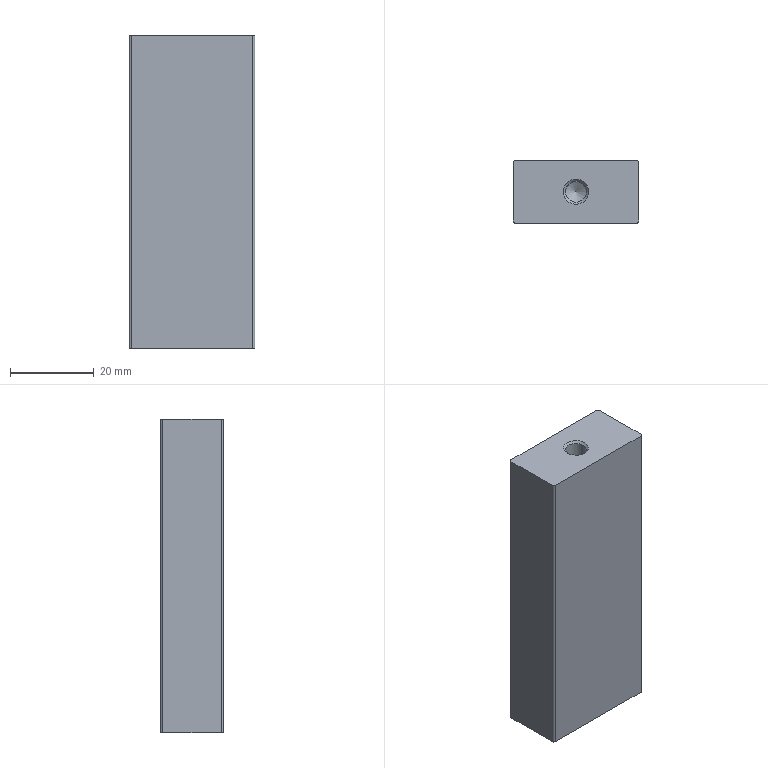Part | STEP file | 200 mesh_id1938 | 1 solid | 13 faces | box 30 x 15 x 75 mm | volume 33075 mm3 | plane 6 | cylinder 5 | cone 2 | commonest cylinder face diameters 1 x4 5 x1
STEP:
#1=CARTESIAN_POINT('',(-16621.224,-4110.769,87.));
#2=VERTEX_POINT('',#1);
#3=CARTESIAN_POINT('',(-16621.224,-4124.769,87.));
#4=VERTEX_POINT('',#3);
#5=CARTESIAN_POINT('',(-16621.224,-4110.769,87.));
#6=DIRECTION('',(0.,-1.,0.));
#7=VECTOR('',#6,1.);
#8=LINE('',#5,#7);
#9=EDGE_CURVE('',#2,#4,#8,.T.);
#10=ORIENTED_EDGE('',*,*,#9,.T.);
#11=CARTESIAN_POINT('',(-16621.224,-4124.769,12.));
#12=VERTEX_POINT('',#11);
#13=CARTESIAN_POINT('',(-16621.224,-4124.769,12.));
#14=DIRECTION('',(0.,0.,1.));
#15=VECTOR('',#14,1.);
#16=LINE('',#13,#15);
#17=EDGE_CURVE('',#12,#4,#16,.T.);
#18=ORIENTED_EDGE('',*,*,#17,.F.);
#19=CARTESIAN_POINT('',(-16621.224,-4110.769,12.));
#20=VERTEX_POINT('',#19);
#21=CARTESIAN_POINT('',(-16621.224,-4110.769,12.));
#22=DIRECTION('',(0.,-1.,0.));
#23=VECTOR('',#22,1.);
#24=LINE('',#21,#23);
#25=EDGE_CURVE('',#20,#12,#24,.T.);
#26=ORIENTED_EDGE('',*,*,#25,.F.);
#27=CARTESIAN_POINT('',(-16621.224,-4110.769,12.));
#28=DIRECTION('',(0.,0.,1.));
#29=VECTOR('',#28,1.);
#30=LINE('',#27,#29);
#31=EDGE_CURVE('',#20,#2,#30,.T.);
#32=ORIENTED_EDGE('',*,*,#31,.T.);
#33=EDGE_LOOP('',(#10,#18,#26,#32));
#34=FACE_OUTER_BOUND('',#33,.T.);
#35=CARTESIAN_POINT('',(-16621.224,-4110.769,12.));
#36=DIRECTION('',(-1.,0.,0.));
#37=DIRECTION('',(0.,-1.,0.));
#38=AXIS2_PLACEMENT_3D('',#35,#36,#37);
#39=PLANE('',#38);
#40=ADVANCED_FACE('',(#34),#39,.F.);
#41=CARTESIAN_POINT('',(-16621.724,-4125.269,87.));
#42=VERTEX_POINT('',#41);
#43=CARTESIAN_POINT('',(-16621.724,-4124.769,87.));
#44=DIRECTION('',(0.,0.,-1.));
#45=DIRECTION('',(1.,0.,0.));
#46=AXIS2_PLACEMENT_3D('',#43,#44,#45);
#47=CIRCLE('',#46,0.5);
#48=EDGE_CURVE('',#4,#42,#47,.T.);
#49=ORIENTED_EDGE('',*,*,#48,.T.);
#50=CARTESIAN_POINT('',(-16621.724,-4125.269,12.));
#51=VERTEX_POINT('',#50);
#52=CARTESIAN_POINT('',(-16621.724,-4125.269,12.));
#53=DIRECTION('',(0.,0.,1.));
#54=VECTOR('',#53,1.);
#55=LINE('',#52,#54);
#56=EDGE_CURVE('',#51,#42,#55,.T.);
#57=ORIENTED_EDGE('',*,*,#56,.F.);
#58=CARTESIAN_POINT('',(-16621.724,-4124.769,12.));
#59=DIRECTION('',(0.,0.,-1.));
#60=DIRECTION('',(1.,0.,0.));
#61=AXIS2_PLACEMENT_3D('',#58,#59,#60);
#62=CIRCLE('',#61,0.5);
#63=EDGE_CURVE('',#12,#51,#62,.T.);
#64=ORIENTED_EDGE('',*,*,#63,.F.);
#65=ORIENTED_EDGE('',*,*,#17,.T.);
#66=EDGE_LOOP('',(#49,#57,#64,#65));
#67=FACE_OUTER_BOUND('',#66,.T.);
#68=CARTESIAN_POINT('',(-16621.724,-4124.769,12.));
#69=DIRECTION('',(0.,0.,1.));
#70=DIRECTION('',(1.,0.,0.));
#71=AXIS2_PLACEMENT_3D('',#68,#69,#70);
#72=CYLINDRICAL_SURFACE('',#71,0.5);
#73=ADVANCED_FACE('',(#67),#72,.T.);
#74=CARTESIAN_POINT('',(-16650.724,-4125.269,87.));
#75=VERTEX_POINT('',#74);
#76=CARTESIAN_POINT('',(-16621.724,-4125.269,87.));
#77=DIRECTION('',(-1.,0.,0.));
#78=VECTOR('',#77,1.);
#79=LINE('',#76,#78);
#80=EDGE_CURVE('',#42,#75,#79,.T.);
#81=ORIENTED_EDGE('',*,*,#80,.T.);
#82=CARTESIAN_POINT('',(-16650.724,-4125.269,12.));
#83=VERTEX_POINT('',#82);
#84=CARTESIAN_POINT('',(-16650.724,-4125.269,12.));
#85=DIRECTION('',(0.,0.,1.));
#86=VECTOR('',#85,1.);
#87=LINE('',#84,#86);
#88=EDGE_CURVE('',#83,#75,#87,.T.);
#89=ORIENTED_EDGE('',*,*,#88,.F.);
#90=CARTESIAN_POINT('',(-16621.724,-4125.269,12.));
#91=DIRECTION('',(-1.,0.,0.));
#92=VECTOR('',#91,1.);
#93=LINE('',#90,#92);
#94=EDGE_CURVE('',#51,#83,#93,.T.);
#95=ORIENTED_EDGE('',*,*,#94,.F.);
#96=ORIENTED_EDGE('',*,*,#56,.T.);
#97=EDGE_LOOP('',(#81,#89,#95,#96));
#98=FACE_OUTER_BOUND('',#97,.T.);
#99=CARTESIAN_POINT('',(-16621.724,-4125.269,12.));
#100=DIRECTION('',(0.,1.,0.));
#101=DIRECTION('',(0.,0.,1.));
#102=AXIS2_PLACEMENT_3D('',#99,#100,#101);
#103=PLANE('',#102);
#104=ADVANCED_FACE('',(#98),#103,.F.);
#105=CARTESIAN_POINT('',(-16651.224,-4124.769,87.));
#106=VERTEX_POINT('',#105);
#107=CARTESIAN_POINT('',(-16650.724,-4124.769,87.));
#108=DIRECTION('',(0.,0.,-1.));
#109=DIRECTION('',(1.,0.,0.));
#110=AXIS2_PLACEMENT_3D('',#107,#108,#109);
#111=CIRCLE('',#110,0.5);
#112=EDGE_CURVE('',#75,#106,#111,.T.);
#113=ORIENTED_EDGE('',*,*,#112,.T.);
#114=CARTESIAN_POINT('',(-16651.224,-4124.769,12.));
#115=VERTEX_POINT('',#114);
#116=CARTESIAN_POINT('',(-16651.224,-4124.769,12.));
#117=DIRECTION('',(0.,0.,1.));
#118=VECTOR('',#117,1.);
#119=LINE('',#116,#118);
#120=EDGE_CURVE('',#115,#106,#119,.T.);
#121=ORIENTED_EDGE('',*,*,#120,.F.);
#122=CARTESIAN_POINT('',(-16650.724,-4124.769,12.));
#123=DIRECTION('',(0.,0.,-1.));
#124=DIRECTION('',(1.,0.,0.));
#125=AXIS2_PLACEMENT_3D('',#122,#123,#124);
#126=CIRCLE('',#125,0.5);
#127=EDGE_CURVE('',#83,#115,#126,.T.);
#128=ORIENTED_EDGE('',*,*,#127,.F.);
#129=ORIENTED_EDGE('',*,*,#88,.T.);
#130=EDGE_LOOP('',(#113,#121,#128,#129));
#131=FACE_OUTER_BOUND('',#130,.T.);
#132=CARTESIAN_POINT('',(-16650.724,-4124.769,12.));
#133=DIRECTION('',(0.,0.,1.));
#134=DIRECTION('',(1.,0.,0.));
#135=AXIS2_PLACEMENT_3D('',#132,#133,#134);
#136=CYLINDRICAL_SURFACE('',#135,0.5);
#137=ADVANCED_FACE('',(#131),#136,.T.);
#138=CARTESIAN_POINT('',(-16651.224,-4110.769,87.));
#139=VERTEX_POINT('',#138);
#140=CARTESIAN_POINT('',(-16651.224,-4124.769,87.));
#141=DIRECTION('',(0.,1.,0.));
#142=VECTOR('',#141,1.);
#143=LINE('',#140,#142);
#144=EDGE_CURVE('',#106,#139,#143,.T.);
#145=ORIENTED_EDGE('',*,*,#144,.T.);
#146=CARTESIAN_POINT('',(-16651.224,-4110.769,12.));
#147=VERTEX_POINT('',#146);
#148=CARTESIAN_POINT('',(-16651.224,-4110.769,12.));
#149=DIRECTION('',(0.,0.,1.));
#150=VECTOR('',#149,1.);
#151=LINE('',#148,#150);
#152=EDGE_CURVE('',#147,#139,#151,.T.);
#153=ORIENTED_EDGE('',*,*,#152,.F.);
#154=CARTESIAN_POINT('',(-16651.224,-4124.769,12.));
#155=DIRECTION('',(0.,1.,0.));
#156=VECTOR('',#155,1.);
#157=LINE('',#154,#156);
#158=EDGE_CURVE('',#115,#147,#157,.T.);
#159=ORIENTED_EDGE('',*,*,#158,.F.);
#160=ORIENTED_EDGE('',*,*,#120,.T.);
#161=EDGE_LOOP('',(#145,#153,#159,#160));
#162=FACE_OUTER_BOUND('',#161,.T.);
#163=CARTESIAN_POINT('',(-16651.224,-4124.769,12.));
#164=DIRECTION('',(1.,0.,0.));
#165=DIRECTION('',(0.,0.,-1.));
#166=AXIS2_PLACEMENT_3D('',#163,#164,#165);
#167=PLANE('',#166);
#168=ADVANCED_FACE('',(#162),#167,.F.);
#169=CARTESIAN_POINT('',(-16650.724,-4110.269,87.));
#170=VERTEX_POINT('',#169);
#171=CARTESIAN_POINT('',(-16650.724,-4110.769,87.));
#172=DIRECTION('',(0.,0.,-1.));
#173=DIRECTION('',(1.,0.,0.));
#174=AXIS2_PLACEMENT_3D('',#171,#172,#173);
#175=CIRCLE('',#174,0.5);
#176=EDGE_CURVE('',#139,#170,#175,.T.);
#177=ORIENTED_EDGE('',*,*,#176,.T.);
#178=CARTESIAN_POINT('',(-16650.724,-4110.269,12.));
#179=VERTEX_POINT('',#178);
#180=CARTESIAN_POINT('',(-16650.724,-4110.269,12.));
#181=DIRECTION('',(0.,0.,1.));
#182=VECTOR('',#181,1.);
#183=LINE('',#180,#182);
#184=EDGE_CURVE('',#179,#170,#183,.T.);
#185=ORIENTED_EDGE('',*,*,#184,.F.);
#186=CARTESIAN_POINT('',(-16650.724,-4110.769,12.));
#187=DIRECTION('',(0.,0.,-1.));
#188=DIRECTION('',(1.,0.,0.));
#189=AXIS2_PLACEMENT_3D('',#186,#187,#188);
#190=CIRCLE('',#189,0.5);
#191=EDGE_CURVE('',#147,#179,#190,.T.);
#192=ORIENTED_EDGE('',*,*,#191,.F.);
#193=ORIENTED_EDGE('',*,*,#152,.T.);
#194=EDGE_LOOP('',(#177,#185,#192,#193));
#195=FACE_OUTER_BOUND('',#194,.T.);
#196=CARTESIAN_POINT('',(-16650.724,-4110.769,12.));
#197=DIRECTION('',(0.,0.,1.));
#198=DIRECTION('',(1.,0.,0.));
#199=AXIS2_PLACEMENT_3D('',#196,#197,#198);
#200=CYLINDRICAL_SURFACE('',#199,0.5);
#201=ADVANCED_FACE('',(#195),#200,.T.);
#202=CARTESIAN_POINT('',(-16621.724,-4110.269,87.));
#203=VERTEX_POINT('',#202);
#204=CARTESIAN_POINT('',(-16650.724,-4110.269,87.));
#205=DIRECTION('',(1.,0.,0.));
#206=VECTOR('',#205,1.);
#207=LINE('',#204,#206);
#208=EDGE_CURVE('',#170,#203,#207,.T.);
#209=ORIENTED_EDGE('',*,*,#208,.T.);
#210=CARTESIAN_POINT('',(-16621.724,-4110.269,12.));
#211=VERTEX_POINT('',#210);
#212=CARTESIAN_POINT('',(-16621.724,-4110.269,12.));
#213=DIRECTION('',(0.,0.,1.));
#214=VECTOR('',#213,1.);
#215=LINE('',#212,#214);
#216=EDGE_CURVE('',#211,#203,#215,.T.);
#217=ORIENTED_EDGE('',*,*,#216,.F.);
#218=CARTESIAN_POINT('',(-16650.724,-4110.269,12.));
#219=DIRECTION('',(1.,0.,0.));
#220=VECTOR('',#219,1.);
#221=LINE('',#218,#220);
#222=EDGE_CURVE('',#179,#211,#221,.T.);
#223=ORIENTED_EDGE('',*,*,#222,.F.);
#224=ORIENTED_EDGE('',*,*,#184,.T.);
#225=EDGE_LOOP('',(#209,#217,#223,#224));
#226=FACE_OUTER_BOUND('',#225,.T.);
#227=CARTESIAN_POINT('',(-16650.724,-4110.269,12.));
#228=DIRECTION('',(0.,-1.,0.));
#229=DIRECTION('',(0.,0.,-1.));
#230=AXIS2_PLACEMENT_3D('',#227,#228,#229);
#231=PLANE('',#230);
#232=ADVANCED_FACE('',(#226),#231,.F.);
#233=CARTESIAN_POINT('',(-16621.724,-4110.769,87.));
#234=DIRECTION('',(0.,0.,-1.));
#235=DIRECTION('',(1.,0.,0.));
#236=AXIS2_PLACEMENT_3D('',#233,#234,#235);
#237=CIRCLE('',#236,0.5);
#238=EDGE_CURVE('',#203,#2,#237,.T.);
#239=ORIENTED_EDGE('',*,*,#238,.T.);
#240=ORIENTED_EDGE('',*,*,#31,.F.);
#241=CARTESIAN_POINT('',(-16621.724,-4110.769,12.));
#242=DIRECTION('',(0.,0.,-1.));
#243=DIRECTION('',(1.,0.,0.));
#244=AXIS2_PLACEMENT_3D('',#241,#242,#243);
#245=CIRCLE('',#244,0.5);
#246=EDGE_CURVE('',#211,#20,#245,.T.);
#247=ORIENTED_EDGE('',*,*,#246,.F.);
#248=ORIENTED_EDGE('',*,*,#216,.T.);
#249=EDGE_LOOP('',(#239,#240,#247,#248));
#250=FACE_OUTER_BOUND('',#249,.T.);
#251=CARTESIAN_POINT('',(-16621.724,-4110.769,12.));
#252=DIRECTION('',(0.,0.,1.));
#253=DIRECTION('',(1.,0.,0.));
#254=AXIS2_PLACEMENT_3D('',#251,#252,#253);
#255=CYLINDRICAL_SURFACE('',#254,0.5);
#256=ADVANCED_FACE('',(#250),#255,.T.);
#257=ORIENTED_EDGE('',*,*,#25,.T.);
#258=ORIENTED_EDGE('',*,*,#63,.T.);
#259=ORIENTED_EDGE('',*,*,#94,.T.);
#260=ORIENTED_EDGE('',*,*,#127,.T.);
#261=ORIENTED_EDGE('',*,*,#158,.T.);
#262=ORIENTED_EDGE('',*,*,#191,.T.);
#263=ORIENTED_EDGE('',*,*,#222,.T.);
#264=ORIENTED_EDGE('',*,*,#246,.T.);
#265=EDGE_LOOP('',(#257,#258,#259,#260,#261,#262,#263,#264));
#266=FACE_OUTER_BOUND('',#265,.T.);
#267=CARTESIAN_POINT('',(-16621.724,-4124.769,12.));
#268=DIRECTION('',(0.,0.,-1.));
#269=DIRECTION('',(-1.,0.,0.));
#270=AXIS2_PLACEMENT_3D('',#267,#268,#269);
#271=PLANE('',#270);
#272=ADVANCED_FACE('',(#266),#271,.T.);
#273=CARTESIAN_POINT('',(-16639.224,-4117.769,87.));
#274=VERTEX_POINT('',#273);
#275=CARTESIAN_POINT('',(-16636.224,-4117.769,87.));
#276=DIRECTION('',(0.,0.,-1.));
#277=DIRECTION('',(-1.,0.,0.));
#278=AXIS2_PLACEMENT_3D('',#275,#276,#277);
#279=CIRCLE('',#278,3.);
#280=EDGE_CURVE('',#274,#274,#279,.T.);
#281=ORIENTED_EDGE('',*,*,#280,.T.);
#282=EDGE_LOOP('',(#281));
#283=FACE_BOUND('',#282,.T.);
#284=ORIENTED_EDGE('',*,*,#9,.F.);
#285=ORIENTED_EDGE('',*,*,#238,.F.);
#286=ORIENTED_EDGE('',*,*,#208,.F.);
#287=ORIENTED_EDGE('',*,*,#176,.F.);
#288=ORIENTED_EDGE('',*,*,#144,.F.);
#289=ORIENTED_EDGE('',*,*,#112,.F.);
#290=ORIENTED_EDGE('',*,*,#80,.F.);
#291=ORIENTED_EDGE('',*,*,#48,.F.);
#292=EDGE_LOOP('',(#284,#285,#286,#287,#288,#289,#290,#291));
#293=FACE_BOUND('',#292,.T.);
#294=CARTESIAN_POINT('',(-16621.724,-4124.769,87.));
#295=DIRECTION('',(0.,0.,-1.));
#296=DIRECTION('',(-1.,0.,0.));
#297=AXIS2_PLACEMENT_3D('',#294,#295,#296);
#298=PLANE('',#297);
#299=ADVANCED_FACE('',(#283,#293),#298,.F.);
#300=CARTESIAN_POINT('',(-16638.724,-4117.769,54.056));
#301=VERTEX_POINT('',#300);
#302=CARTESIAN_POINT('',(-16636.224,-4117.769,54.056));
#303=DIRECTION('',(0.,0.,1.));
#304=DIRECTION('',(-1.,0.,0.));
#305=AXIS2_PLACEMENT_3D('',#302,#303,#304);
#306=CIRCLE('',#305,2.5);
#307=EDGE_CURVE('',#301,#301,#306,.T.);
#308=ORIENTED_EDGE('',*,*,#307,.T.);
#309=EDGE_LOOP('',(#308));
#310=FACE_BOUND('',#309,.T.);
#311=CARTESIAN_POINT('',(-16636.224,-4117.769,52.554));
#312=VERTEX_POINT('',#311);
#313=VERTEX_LOOP('',#312);
#314=FACE_BOUND('',#313,.T.);
#315=CARTESIAN_POINT('',(-16636.224,-4117.769,54.056));
#316=DIRECTION('',(0.,0.,1.));
#317=DIRECTION('',(1.,0.,0.));
#318=AXIS2_PLACEMENT_3D('',#315,#316,#317);
#319=CONICAL_SURFACE('',#318,2.5,59.);
#320=ADVANCED_FACE('',(#310,#314),#319,.F.);
#321=CARTESIAN_POINT('',(-16638.724,-4117.769,86.5));
#322=VERTEX_POINT('',#321);
#323=CARTESIAN_POINT('',(-16636.224,-4117.769,86.5));
#324=DIRECTION('',(0.,0.,1.));
#325=DIRECTION('',(-1.,0.,0.));
#326=AXIS2_PLACEMENT_3D('',#323,#324,#325);
#327=CIRCLE('',#326,2.5);
#328=EDGE_CURVE('',#322,#322,#327,.T.);
#329=ORIENTED_EDGE('',*,*,#328,.T.);
#330=EDGE_LOOP('',(#329));
#331=FACE_BOUND('',#330,.T.);
#332=ORIENTED_EDGE('',*,*,#307,.F.);
#333=EDGE_LOOP('',(#332));
#334=FACE_BOUND('',#333,.T.);
#335=CARTESIAN_POINT('',(-16636.224,-4117.769,89.056));
#336=DIRECTION('',(0.,0.,-1.));
#337=DIRECTION('',(-1.,0.,0.));
#338=AXIS2_PLACEMENT_3D('',#335,#336,#337);
#339=CYLINDRICAL_SURFACE('',#338,2.5);
#340=ADVANCED_FACE('',(#331,#334),#339,.F.);
#341=ORIENTED_EDGE('',*,*,#328,.F.);
#342=EDGE_LOOP('',(#341));
#343=FACE_BOUND('',#342,.T.);
#344=ORIENTED_EDGE('',*,*,#280,.F.);
#345=EDGE_LOOP('',(#344));
#346=FACE_BOUND('',#345,.T.);
#347=CARTESIAN_POINT('',(-16636.224,-4117.769,87.));
#348=DIRECTION('',(0.,0.,1.));
#349=DIRECTION('',(1.,0.,0.));
#350=AXIS2_PLACEMENT_3D('',#347,#348,#349);
#351=CONICAL_SURFACE('',#350,3.,45.);
#352=ADVANCED_FACE('',(#343,#346),#351,.F.);
#353=CLOSED_SHELL('',(#40,#73,#104,#137,#168,#201,#232,#256,#272,#299,#320,#340,#352));
#354=MANIFOLD_SOLID_BREP('',#353);
#355=(LENGTH_UNIT()NAMED_UNIT(*)SI_UNIT(.MILLI.,.METRE.));
#356=UNCERTAINTY_MEASURE_WITH_UNIT(LENGTH_MEASURE(0.00002),#355,'','');
#357=(NAMED_UNIT(*)PLANE_ANGLE_UNIT()SI_UNIT($,.RADIAN.));
#358=PLANE_ANGLE_MEASURE_WITH_UNIT(PLANE_ANGLE_MEASURE(0.01745),#357);
#359=DIMENSIONAL_EXPONENTS(0.,0.,0.,0.,0.,0.,0.);
#360=(CONVERSION_BASED_UNIT('DEGREE',#358)NAMED_UNIT(#359)PLANE_ANGLE_UNIT());
#361=(NAMED_UNIT(*)SI_UNIT($,.STERADIAN.)SOLID_ANGLE_UNIT());
#362=(GEOMETRIC_REPRESENTATION_CONTEXT(3)GLOBAL_UNCERTAINTY_ASSIGNED_CONTEXT((#356))GLOBAL_UNIT_ASSIGNED_CONTEXT((#355,#360,#361))REPRESENTATION_CONTEXT('',''));
#363=ADVANCED_BREP_SHAPE_REPRESENTATION('',(#354),#362);